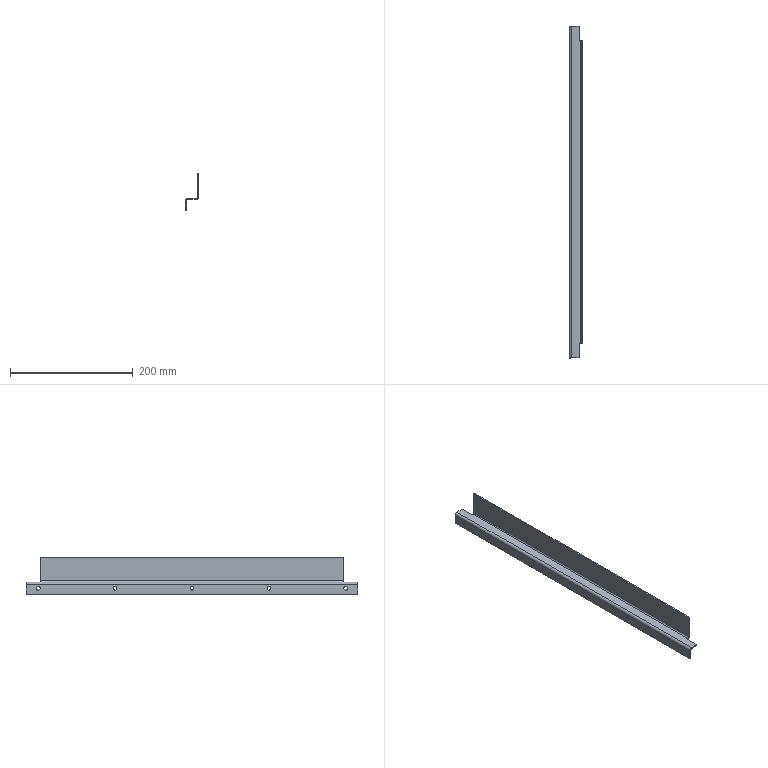Part | NX | features solid 2 | 1 solid | 28 faces | box 22 x 540 x 60 mm | volume 79205 mm3 | plane 14 | cylinder 14 | commonest cylinder face diameters 6 x10 4 x2 8 x2
STEP:
#1=CARTESIAN_POINT('',(-1090.,-1270.9,118.));
#2=VERTEX_POINT('',#1);
#3=CARTESIAN_POINT('',(-1092.,-1270.9,118.));
#4=VERTEX_POINT('',#3);
#5=CARTESIAN_POINT('',(-1108.,-1270.9,118.));
#6=DIRECTION('',(-1.,0.,0.));
#7=VECTOR('',#6,1000.);
#8=LINE('',#5,#7);
#9=EDGE_CURVE('',#2,#4,#8,.T.);
#10=ORIENTED_EDGE('',*,*,#9,.F.);
#11=CARTESIAN_POINT('',(-1086.,-1270.9,122.));
#12=VERTEX_POINT('',#11);
#13=CARTESIAN_POINT('',(-1090.,-1270.9,122.));
#14=DIRECTION('',(0.,1.,0.));
#15=DIRECTION('',(0.,0.,-1.));
#16=AXIS2_PLACEMENT_3D('',#13,#14,#15);
#17=CIRCLE('',#16,4.);
#18=EDGE_CURVE('',#12,#2,#17,.T.);
#19=ORIENTED_EDGE('',*,*,#18,.F.);
#20=CARTESIAN_POINT('',(-1086.,-1270.9,160.));
#21=VERTEX_POINT('',#20);
#22=CARTESIAN_POINT('',(-1086.,-1270.9,120.));
#23=DIRECTION('',(0.,0.,-1.));
#24=VECTOR('',#23,1000.);
#25=LINE('',#22,#24);
#26=EDGE_CURVE('',#21,#12,#25,.T.);
#27=ORIENTED_EDGE('',*,*,#26,.F.);
#28=CARTESIAN_POINT('',(-1088.,-1270.9,160.));
#29=VERTEX_POINT('',#28);
#30=CARTESIAN_POINT('',(-1088.,-1270.9,160.));
#31=DIRECTION('',(-1.,0.,0.));
#32=VECTOR('',#31,1000.);
#33=LINE('',#30,#32);
#34=EDGE_CURVE('',#21,#29,#33,.T.);
#35=ORIENTED_EDGE('',*,*,#34,.T.);
#36=CARTESIAN_POINT('',(-1088.,-1270.9,122.));
#37=VERTEX_POINT('',#36);
#38=CARTESIAN_POINT('',(-1088.,-1270.9,120.));
#39=DIRECTION('',(0.,0.,-1.));
#40=VECTOR('',#39,1000.);
#41=LINE('',#38,#40);
#42=EDGE_CURVE('',#29,#37,#41,.T.);
#43=ORIENTED_EDGE('',*,*,#42,.T.);
#44=CARTESIAN_POINT('',(-1090.,-1270.9,120.));
#45=VERTEX_POINT('',#44);
#46=CARTESIAN_POINT('',(-1090.,-1270.9,122.));
#47=DIRECTION('',(0.,1.,0.));
#48=DIRECTION('',(0.,0.,-1.));
#49=AXIS2_PLACEMENT_3D('',#46,#47,#48);
#50=CIRCLE('',#49,2.);
#51=EDGE_CURVE('',#37,#45,#50,.T.);
#52=ORIENTED_EDGE('',*,*,#51,.T.);
#53=CARTESIAN_POINT('',(-1092.,-1270.9,120.));
#54=VERTEX_POINT('',#53);
#55=CARTESIAN_POINT('',(-1108.,-1270.9,120.));
#56=DIRECTION('',(-1.,0.,0.));
#57=VECTOR('',#56,1000.);
#58=LINE('',#55,#57);
#59=EDGE_CURVE('',#45,#54,#58,.T.);
#60=ORIENTED_EDGE('',*,*,#59,.T.);
#61=CARTESIAN_POINT('',(-1092.,-1270.9,120.));
#62=DIRECTION('',(0.,0.,1.));
#63=VECTOR('',#62,1000.);
#64=LINE('',#61,#63);
#65=EDGE_CURVE('',#4,#54,#64,.T.);
#66=ORIENTED_EDGE('',*,*,#65,.F.);
#67=EDGE_LOOP('',(#10,#19,#27,#35,#43,#52,#60,#66));
#68=FACE_BOUND('',#67,.T.);
#69=CARTESIAN_POINT('',(-1108.,-1270.9,120.));
#70=DIRECTION('',(0.,1.,0.));
#71=DIRECTION('',(0.,0.,-1.));
#72=AXIS2_PLACEMENT_3D('',#69,#70,#71);
#73=PLANE('',#72);
#74=ADVANCED_FACE('',(#68),#73,.F.);
#75=ORIENTED_EDGE('',*,*,#65,.T.);
#76=CARTESIAN_POINT('',(-1092.,-1294.,120.));
#77=VERTEX_POINT('',#76);
#78=CARTESIAN_POINT('',(-1092.,-1294.,120.));
#79=DIRECTION('',(0.,1.,0.));
#80=VECTOR('',#79,1000.);
#81=LINE('',#78,#80);
#82=EDGE_CURVE('',#77,#54,#81,.T.);
#83=ORIENTED_EDGE('',*,*,#82,.F.);
#84=CARTESIAN_POINT('',(-1092.,-1294.,118.));
#85=VERTEX_POINT('',#84);
#86=CARTESIAN_POINT('',(-1092.,-1294.,120.));
#87=DIRECTION('',(0.,0.,1.));
#88=VECTOR('',#87,1000.);
#89=LINE('',#86,#88);
#90=EDGE_CURVE('',#85,#77,#89,.T.);
#91=ORIENTED_EDGE('',*,*,#90,.F.);
#92=CARTESIAN_POINT('',(-1092.,-1294.,118.));
#93=DIRECTION('',(0.,1.,0.));
#94=VECTOR('',#93,1000.);
#95=LINE('',#92,#94);
#96=EDGE_CURVE('',#85,#4,#95,.T.);
#97=ORIENTED_EDGE('',*,*,#96,.T.);
#98=EDGE_LOOP('',(#75,#83,#91,#97));
#99=FACE_BOUND('',#98,.T.);
#100=CARTESIAN_POINT('',(-1092.,-1294.,120.));
#101=DIRECTION('',(1.,0.,0.));
#102=DIRECTION('',(0.,0.,-1.));
#103=AXIS2_PLACEMENT_3D('',#100,#101,#102);
#104=PLANE('',#103);
#105=ADVANCED_FACE('',(#99),#104,.T.);
#106=CARTESIAN_POINT('',(-1086.,-777.1,122.));
#107=VERTEX_POINT('',#106);
#108=CARTESIAN_POINT('',(-1086.,-777.1,160.));
#109=VERTEX_POINT('',#108);
#110=CARTESIAN_POINT('',(-1086.,-777.1,120.));
#111=DIRECTION('',(0.,0.,1.));
#112=VECTOR('',#111,1000.);
#113=LINE('',#110,#112);
#114=EDGE_CURVE('',#107,#109,#113,.T.);
#115=ORIENTED_EDGE('',*,*,#114,.F.);
#116=CARTESIAN_POINT('',(-1090.,-777.1,118.));
#117=VERTEX_POINT('',#116);
#118=CARTESIAN_POINT('',(-1090.,-777.1,122.));
#119=DIRECTION('',(0.,-1.,0.));
#120=DIRECTION('',(0.,0.,-1.));
#121=AXIS2_PLACEMENT_3D('',#118,#119,#120);
#122=CIRCLE('',#121,4.);
#123=EDGE_CURVE('',#117,#107,#122,.T.);
#124=ORIENTED_EDGE('',*,*,#123,.F.);
#125=CARTESIAN_POINT('',(-1092.,-777.1,118.));
#126=VERTEX_POINT('',#125);
#127=CARTESIAN_POINT('',(-1108.,-777.1,118.));
#128=DIRECTION('',(1.,0.,0.));
#129=VECTOR('',#128,1000.);
#130=LINE('',#127,#129);
#131=EDGE_CURVE('',#126,#117,#130,.T.);
#132=ORIENTED_EDGE('',*,*,#131,.F.);
#133=CARTESIAN_POINT('',(-1092.,-777.1,120.));
#134=VERTEX_POINT('',#133);
#135=CARTESIAN_POINT('',(-1092.,-777.1,120.));
#136=DIRECTION('',(0.,0.,1.));
#137=VECTOR('',#136,1000.);
#138=LINE('',#135,#137);
#139=EDGE_CURVE('',#126,#134,#138,.T.);
#140=ORIENTED_EDGE('',*,*,#139,.T.);
#141=CARTESIAN_POINT('',(-1090.,-777.1,120.));
#142=VERTEX_POINT('',#141);
#143=CARTESIAN_POINT('',(-1108.,-777.1,120.));
#144=DIRECTION('',(1.,0.,0.));
#145=VECTOR('',#144,1000.);
#146=LINE('',#143,#145);
#147=EDGE_CURVE('',#134,#142,#146,.T.);
#148=ORIENTED_EDGE('',*,*,#147,.T.);
#149=CARTESIAN_POINT('',(-1088.,-777.1,122.));
#150=VERTEX_POINT('',#149);
#151=CARTESIAN_POINT('',(-1090.,-777.1,122.));
#152=DIRECTION('',(0.,-1.,0.));
#153=DIRECTION('',(0.,0.,1.));
#154=AXIS2_PLACEMENT_3D('',#151,#152,#153);
#155=CIRCLE('',#154,2.);
#156=EDGE_CURVE('',#142,#150,#155,.T.);
#157=ORIENTED_EDGE('',*,*,#156,.T.);
#158=CARTESIAN_POINT('',(-1088.,-777.1,160.));
#159=VERTEX_POINT('',#158);
#160=CARTESIAN_POINT('',(-1088.,-777.1,120.));
#161=DIRECTION('',(0.,0.,1.));
#162=VECTOR('',#161,1000.);
#163=LINE('',#160,#162);
#164=EDGE_CURVE('',#150,#159,#163,.T.);
#165=ORIENTED_EDGE('',*,*,#164,.T.);
#166=CARTESIAN_POINT('',(-1088.,-777.1,160.));
#167=DIRECTION('',(-1.,0.,0.));
#168=VECTOR('',#167,1000.);
#169=LINE('',#166,#168);
#170=EDGE_CURVE('',#109,#159,#169,.T.);
#171=ORIENTED_EDGE('',*,*,#170,.F.);
#172=EDGE_LOOP('',(#115,#124,#132,#140,#148,#157,#165,#171));
#173=FACE_BOUND('',#172,.T.);
#174=CARTESIAN_POINT('',(-1088.,-777.1,120.));
#175=DIRECTION('',(0.,-1.,0.));
#176=DIRECTION('',(-1.,0.,0.));
#177=AXIS2_PLACEMENT_3D('',#174,#175,#176);
#178=PLANE('',#177);
#179=ADVANCED_FACE('',(#173),#178,.F.);
#180=CARTESIAN_POINT('',(-1092.,-754.,118.));
#181=VERTEX_POINT('',#180);
#182=CARTESIAN_POINT('',(-1092.,-754.,120.));
#183=VERTEX_POINT('',#182);
#184=CARTESIAN_POINT('',(-1092.,-754.,120.));
#185=DIRECTION('',(0.,0.,1.));
#186=VECTOR('',#185,1000.);
#187=LINE('',#184,#186);
#188=EDGE_CURVE('',#181,#183,#187,.T.);
#189=ORIENTED_EDGE('',*,*,#188,.T.);
#190=CARTESIAN_POINT('',(-1092.,-1294.,120.));
#191=DIRECTION('',(0.,1.,0.));
#192=VECTOR('',#191,1000.);
#193=LINE('',#190,#192);
#194=EDGE_CURVE('',#134,#183,#193,.T.);
#195=ORIENTED_EDGE('',*,*,#194,.F.);
#196=ORIENTED_EDGE('',*,*,#139,.F.);
#197=CARTESIAN_POINT('',(-1092.,-1294.,118.));
#198=DIRECTION('',(0.,1.,0.));
#199=VECTOR('',#198,1000.);
#200=LINE('',#197,#199);
#201=EDGE_CURVE('',#126,#181,#200,.T.);
#202=ORIENTED_EDGE('',*,*,#201,.T.);
#203=EDGE_LOOP('',(#189,#195,#196,#202));
#204=FACE_BOUND('',#203,.T.);
#205=CARTESIAN_POINT('',(-1092.,-1294.,120.));
#206=DIRECTION('',(1.,0.,0.));
#207=DIRECTION('',(0.,0.,-1.));
#208=AXIS2_PLACEMENT_3D('',#205,#206,#207);
#209=PLANE('',#208);
#210=ADVANCED_FACE('',(#204),#209,.T.);
#211=CARTESIAN_POINT('',(-1108.,-1024.,107.));
#212=VERTEX_POINT('',#211);
#213=CARTESIAN_POINT('',(-1106.,-1024.,107.));
#214=VERTEX_POINT('',#213);
#215=CARTESIAN_POINT('',(-1649.768,-1024.,107.));
#216=DIRECTION('',(1.,0.,0.));
#217=VECTOR('',#216,1000.);
#218=LINE('',#215,#217);
#219=EDGE_CURVE('',#212,#214,#218,.T.);
#220=ORIENTED_EDGE('',*,*,#219,.F.);
#221=CARTESIAN_POINT('',(-1108.,-1024.,113.));
#222=VERTEX_POINT('',#221);
#223=CARTESIAN_POINT('',(-1108.,-1024.,110.));
#224=DIRECTION('',(-1.,0.,0.));
#225=DIRECTION('',(0.,0.,-1.));
#226=AXIS2_PLACEMENT_3D('',#223,#224,#225);
#227=CIRCLE('',#226,3.);
#228=EDGE_CURVE('',#212,#222,#227,.T.);
#229=ORIENTED_EDGE('',*,*,#228,.T.);
#230=CARTESIAN_POINT('',(-1106.,-1024.,113.));
#231=VERTEX_POINT('',#230);
#232=CARTESIAN_POINT('',(-1649.768,-1024.,113.));
#233=DIRECTION('',(1.,0.,0.));
#234=VECTOR('',#233,1000.);
#235=LINE('',#232,#234);
#236=EDGE_CURVE('',#231,#222,#235,.F.);
#237=ORIENTED_EDGE('',*,*,#236,.F.);
#238=CARTESIAN_POINT('',(-1106.,-1024.,110.));
#239=DIRECTION('',(1.,0.,0.));
#240=DIRECTION('',(0.,1.,0.));
#241=AXIS2_PLACEMENT_3D('',#238,#239,#240);
#242=CIRCLE('',#241,3.);
#243=EDGE_CURVE('',#231,#214,#242,.T.);
#244=ORIENTED_EDGE('',*,*,#243,.T.);
#245=EDGE_LOOP('',(#220,#229,#237,#244));
#246=FACE_BOUND('',#245,.T.);
#247=CARTESIAN_POINT('',(-1649.768,-1024.,110.));
#248=DIRECTION('',(1.,0.,0.));
#249=DIRECTION('',(0.,0.,1.));
#250=AXIS2_PLACEMENT_3D('',#247,#248,#249);
#251=CYLINDRICAL_SURFACE('',#250,3.);
#252=ADVANCED_FACE('',(#246),#251,.F.);
#253=CARTESIAN_POINT('',(-1108.,-1274.,107.));
#254=VERTEX_POINT('',#253);
#255=CARTESIAN_POINT('',(-1106.,-1274.,107.));
#256=VERTEX_POINT('',#255);
#257=CARTESIAN_POINT('',(-1649.768,-1274.,107.));
#258=DIRECTION('',(1.,0.,0.));
#259=VECTOR('',#258,1000.);
#260=LINE('',#257,#259);
#261=EDGE_CURVE('',#254,#256,#260,.T.);
#262=ORIENTED_EDGE('',*,*,#261,.F.);
#263=CARTESIAN_POINT('',(-1108.,-1274.,113.));
#264=VERTEX_POINT('',#263);
#265=CARTESIAN_POINT('',(-1108.,-1274.,110.));
#266=DIRECTION('',(-1.,0.,0.));
#267=DIRECTION('',(0.,0.,-1.));
#268=AXIS2_PLACEMENT_3D('',#265,#266,#267);
#269=CIRCLE('',#268,3.);
#270=EDGE_CURVE('',#254,#264,#269,.T.);
#271=ORIENTED_EDGE('',*,*,#270,.T.);
#272=CARTESIAN_POINT('',(-1106.,-1274.,113.));
#273=VERTEX_POINT('',#272);
#274=CARTESIAN_POINT('',(-1649.768,-1274.,113.));
#275=DIRECTION('',(1.,0.,0.));
#276=VECTOR('',#275,1000.);
#277=LINE('',#274,#276);
#278=EDGE_CURVE('',#273,#264,#277,.F.);
#279=ORIENTED_EDGE('',*,*,#278,.F.);
#280=CARTESIAN_POINT('',(-1106.,-1274.,110.));
#281=DIRECTION('',(1.,0.,0.));
#282=DIRECTION('',(0.,1.,0.));
#283=AXIS2_PLACEMENT_3D('',#280,#281,#282);
#284=CIRCLE('',#283,3.);
#285=EDGE_CURVE('',#273,#256,#284,.T.);
#286=ORIENTED_EDGE('',*,*,#285,.T.);
#287=EDGE_LOOP('',(#262,#271,#279,#286));
#288=FACE_BOUND('',#287,.T.);
#289=CARTESIAN_POINT('',(-1649.768,-1274.,110.));
#290=DIRECTION('',(1.,0.,0.));
#291=DIRECTION('',(0.,0.,1.));
#292=AXIS2_PLACEMENT_3D('',#289,#290,#291);
#293=CYLINDRICAL_SURFACE('',#292,3.);
#294=ADVANCED_FACE('',(#288),#293,.F.);
#295=CARTESIAN_POINT('',(-1106.,-1149.,107.));
#296=VERTEX_POINT('',#295);
#297=CARTESIAN_POINT('',(-1108.,-1149.,107.));
#298=VERTEX_POINT('',#297);
#299=CARTESIAN_POINT('',(-1649.768,-1149.,107.));
#300=DIRECTION('',(1.,0.,0.));
#301=VECTOR('',#300,1000.);
#302=LINE('',#299,#301);
#303=EDGE_CURVE('',#296,#298,#302,.F.);
#304=ORIENTED_EDGE('',*,*,#303,.T.);
#305=CARTESIAN_POINT('',(-1108.,-1149.,113.));
#306=VERTEX_POINT('',#305);
#307=CARTESIAN_POINT('',(-1108.,-1149.,110.));
#308=DIRECTION('',(-1.,0.,0.));
#309=DIRECTION('',(0.,0.,-1.));
#310=AXIS2_PLACEMENT_3D('',#307,#308,#309);
#311=CIRCLE('',#310,3.);
#312=EDGE_CURVE('',#298,#306,#311,.T.);
#313=ORIENTED_EDGE('',*,*,#312,.T.);
#314=CARTESIAN_POINT('',(-1106.,-1149.,113.));
#315=VERTEX_POINT('',#314);
#316=CARTESIAN_POINT('',(-1649.768,-1149.,113.));
#317=DIRECTION('',(1.,0.,0.));
#318=VECTOR('',#317,1000.);
#319=LINE('',#316,#318);
#320=EDGE_CURVE('',#306,#315,#319,.T.);
#321=ORIENTED_EDGE('',*,*,#320,.T.);
#322=CARTESIAN_POINT('',(-1106.,-1149.,110.));
#323=DIRECTION('',(1.,0.,0.));
#324=DIRECTION('',(0.,1.,0.));
#325=AXIS2_PLACEMENT_3D('',#322,#323,#324);
#326=CIRCLE('',#325,3.);
#327=EDGE_CURVE('',#315,#296,#326,.T.);
#328=ORIENTED_EDGE('',*,*,#327,.T.);
#329=EDGE_LOOP('',(#304,#313,#321,#328));
#330=FACE_BOUND('',#329,.T.);
#331=CARTESIAN_POINT('',(-1649.768,-1149.,110.));
#332=DIRECTION('',(1.,0.,0.));
#333=DIRECTION('',(0.,0.,1.));
#334=AXIS2_PLACEMENT_3D('',#331,#332,#333);
#335=CYLINDRICAL_SURFACE('',#334,3.);
#336=ADVANCED_FACE('',(#330),#335,.F.);
#337=CARTESIAN_POINT('',(-1108.,-774.,107.));
#338=VERTEX_POINT('',#337);
#339=CARTESIAN_POINT('',(-1106.,-774.,107.));
#340=VERTEX_POINT('',#339);
#341=CARTESIAN_POINT('',(-1649.768,-774.,107.));
#342=DIRECTION('',(1.,0.,0.));
#343=VECTOR('',#342,1000.);
#344=LINE('',#341,#343);
#345=EDGE_CURVE('',#338,#340,#344,.T.);
#346=ORIENTED_EDGE('',*,*,#345,.F.);
#347=CARTESIAN_POINT('',(-1108.,-774.,113.));
#348=VERTEX_POINT('',#347);
#349=CARTESIAN_POINT('',(-1108.,-774.,110.));
#350=DIRECTION('',(-1.,0.,0.));
#351=DIRECTION('',(0.,0.,-1.));
#352=AXIS2_PLACEMENT_3D('',#349,#350,#351);
#353=CIRCLE('',#352,3.);
#354=EDGE_CURVE('',#338,#348,#353,.T.);
#355=ORIENTED_EDGE('',*,*,#354,.T.);
#356=CARTESIAN_POINT('',(-1106.,-774.,113.));
#357=VERTEX_POINT('',#356);
#358=CARTESIAN_POINT('',(-1649.768,-774.,113.));
#359=DIRECTION('',(1.,0.,0.));
#360=VECTOR('',#359,1000.);
#361=LINE('',#358,#360);
#362=EDGE_CURVE('',#357,#348,#361,.F.);
#363=ORIENTED_EDGE('',*,*,#362,.F.);
#364=CARTESIAN_POINT('',(-1106.,-774.,110.));
#365=DIRECTION('',(1.,0.,0.));
#366=DIRECTION('',(0.,1.,0.));
#367=AXIS2_PLACEMENT_3D('',#364,#365,#366);
#368=CIRCLE('',#367,3.);
#369=EDGE_CURVE('',#357,#340,#368,.T.);
#370=ORIENTED_EDGE('',*,*,#369,.T.);
#371=EDGE_LOOP('',(#346,#355,#363,#370));
#372=FACE_BOUND('',#371,.T.);
#373=CARTESIAN_POINT('',(-1649.768,-774.,110.));
#374=DIRECTION('',(1.,0.,0.));
#375=DIRECTION('',(0.,0.,1.));
#376=AXIS2_PLACEMENT_3D('',#373,#374,#375);
#377=CYLINDRICAL_SURFACE('',#376,3.);
#378=ADVANCED_FACE('',(#372),#377,.F.);
#379=CARTESIAN_POINT('',(-1108.,-899.,107.));
#380=VERTEX_POINT('',#379);
#381=CARTESIAN_POINT('',(-1106.,-899.,107.));
#382=VERTEX_POINT('',#381);
#383=CARTESIAN_POINT('',(-1649.768,-899.,107.));
#384=DIRECTION('',(1.,0.,0.));
#385=VECTOR('',#384,1000.);
#386=LINE('',#383,#385);
#387=EDGE_CURVE('',#380,#382,#386,.T.);
#388=ORIENTED_EDGE('',*,*,#387,.F.);
#389=CARTESIAN_POINT('',(-1108.,-899.,113.));
#390=VERTEX_POINT('',#389);
#391=CARTESIAN_POINT('',(-1108.,-899.,110.));
#392=DIRECTION('',(-1.,0.,0.));
#393=DIRECTION('',(0.,0.,-1.));
#394=AXIS2_PLACEMENT_3D('',#391,#392,#393);
#395=CIRCLE('',#394,3.);
#396=EDGE_CURVE('',#380,#390,#395,.T.);
#397=ORIENTED_EDGE('',*,*,#396,.T.);
#398=CARTESIAN_POINT('',(-1106.,-899.,113.));
#399=VERTEX_POINT('',#398);
#400=CARTESIAN_POINT('',(-1649.768,-899.,113.));
#401=DIRECTION('',(1.,0.,0.));
#402=VECTOR('',#401,1000.);
#403=LINE('',#400,#402);
#404=EDGE_CURVE('',#399,#390,#403,.F.);
#405=ORIENTED_EDGE('',*,*,#404,.F.);
#406=CARTESIAN_POINT('',(-1106.,-899.,110.));
#407=DIRECTION('',(1.,0.,0.));
#408=DIRECTION('',(0.,1.,0.));
#409=AXIS2_PLACEMENT_3D('',#406,#407,#408);
#410=CIRCLE('',#409,3.);
#411=EDGE_CURVE('',#399,#382,#410,.T.);
#412=ORIENTED_EDGE('',*,*,#411,.T.);
#413=EDGE_LOOP('',(#388,#397,#405,#412));
#414=FACE_BOUND('',#413,.T.);
#415=CARTESIAN_POINT('',(-1649.768,-899.,110.));
#416=DIRECTION('',(1.,0.,0.));
#417=DIRECTION('',(0.,0.,1.));
#418=AXIS2_PLACEMENT_3D('',#415,#416,#417);
#419=CYLINDRICAL_SURFACE('',#418,3.);
#420=ADVANCED_FACE('',(#414),#419,.F.);
#421=CARTESIAN_POINT('',(-1086.,-1294.,160.));
#422=DIRECTION('',(0.,1.,0.));
#423=VECTOR('',#422,1000.);
#424=LINE('',#421,#423);
#425=EDGE_CURVE('',#21,#109,#424,.T.);
#426=ORIENTED_EDGE('',*,*,#425,.F.);
#427=ORIENTED_EDGE('',*,*,#26,.T.);
#428=CARTESIAN_POINT('',(-1086.,-1294.,122.));
#429=DIRECTION('',(0.,1.,0.));
#430=VECTOR('',#429,1000.);
#431=LINE('',#428,#430);
#432=EDGE_CURVE('',#12,#107,#431,.T.);
#433=ORIENTED_EDGE('',*,*,#432,.T.);
#434=ORIENTED_EDGE('',*,*,#114,.T.);
#435=EDGE_LOOP('',(#426,#427,#433,#434));
#436=FACE_BOUND('',#435,.T.);
#437=CARTESIAN_POINT('',(-1086.,-1294.,120.));
#438=DIRECTION('',(-1.,0.,0.));
#439=DIRECTION('',(0.,1.,0.));
#440=AXIS2_PLACEMENT_3D('',#437,#438,#439);
#441=PLANE('',#440);
#442=ADVANCED_FACE('',(#436),#441,.F.);
#443=ORIENTED_EDGE('',*,*,#432,.F.);
#444=ORIENTED_EDGE('',*,*,#18,.T.);
#445=CARTESIAN_POINT('',(-1090.,-1294.,118.));
#446=DIRECTION('',(0.,1.,0.));
#447=VECTOR('',#446,1000.);
#448=LINE('',#445,#447);
#449=EDGE_CURVE('',#2,#117,#448,.T.);
#450=ORIENTED_EDGE('',*,*,#449,.T.);
#451=ORIENTED_EDGE('',*,*,#123,.T.);
#452=EDGE_LOOP('',(#443,#444,#450,#451));
#453=FACE_BOUND('',#452,.T.);
#454=CARTESIAN_POINT('',(-1090.,-1294.,122.));
#455=DIRECTION('',(0.,1.,0.));
#456=DIRECTION('',(0.,0.,-1.));
#457=AXIS2_PLACEMENT_3D('',#454,#455,#456);
#458=CYLINDRICAL_SURFACE('',#457,4.);
#459=ADVANCED_FACE('',(#453),#458,.T.);
#460=ORIENTED_EDGE('',*,*,#9,.T.);
#461=ORIENTED_EDGE('',*,*,#96,.F.);
#462=CARTESIAN_POINT('',(-1104.,-1294.,118.));
#463=VERTEX_POINT('',#462);
#464=CARTESIAN_POINT('',(-1108.,-1294.,118.));
#465=DIRECTION('',(1.,0.,0.));
#466=VECTOR('',#465,1000.);
#467=LINE('',#464,#466);
#468=EDGE_CURVE('',#463,#85,#467,.T.);
#469=ORIENTED_EDGE('',*,*,#468,.F.);
#470=CARTESIAN_POINT('',(-1104.,-754.,118.));
#471=VERTEX_POINT('',#470);
#472=CARTESIAN_POINT('',(-1104.,-1294.,118.));
#473=DIRECTION('',(0.,1.,0.));
#474=VECTOR('',#473,1000.);
#475=LINE('',#472,#474);
#476=EDGE_CURVE('',#463,#471,#475,.T.);
#477=ORIENTED_EDGE('',*,*,#476,.T.);
#478=CARTESIAN_POINT('',(-1108.,-754.,118.));
#479=DIRECTION('',(1.,0.,0.));
#480=VECTOR('',#479,1000.);
#481=LINE('',#478,#480);
#482=EDGE_CURVE('',#471,#181,#481,.T.);
#483=ORIENTED_EDGE('',*,*,#482,.T.);
#484=ORIENTED_EDGE('',*,*,#201,.F.);
#485=ORIENTED_EDGE('',*,*,#131,.T.);
#486=ORIENTED_EDGE('',*,*,#449,.F.);
#487=EDGE_LOOP('',(#460,#461,#469,#477,#483,#484,#485,#486));
#488=FACE_BOUND('',#487,.T.);
#489=CARTESIAN_POINT('',(-1108.,-1294.,118.));
#490=DIRECTION('',(0.,0.,1.));
#491=DIRECTION('',(0.,-1.,0.));
#492=AXIS2_PLACEMENT_3D('',#489,#490,#491);
#493=PLANE('',#492);
#494=ADVANCED_FACE('',(#488),#493,.F.);
#495=CARTESIAN_POINT('',(-1106.,-754.,116.));
#496=VERTEX_POINT('',#495);
#497=CARTESIAN_POINT('',(-1104.,-754.,116.));
#498=DIRECTION('',(0.,1.,0.));
#499=DIRECTION('',(0.,0.,-1.));
#500=AXIS2_PLACEMENT_3D('',#497,#498,#499);
#501=CIRCLE('',#500,2.);
#502=EDGE_CURVE('',#496,#471,#501,.T.);
#503=ORIENTED_EDGE('',*,*,#502,.T.);
#504=ORIENTED_EDGE('',*,*,#476,.F.);
#505=CARTESIAN_POINT('',(-1106.,-1294.,116.));
#506=VERTEX_POINT('',#505);
#507=CARTESIAN_POINT('',(-1104.,-1294.,116.));
#508=DIRECTION('',(0.,1.,0.));
#509=DIRECTION('',(0.,0.,-1.));
#510=AXIS2_PLACEMENT_3D('',#507,#508,#509);
#511=CIRCLE('',#510,2.);
#512=EDGE_CURVE('',#506,#463,#511,.T.);
#513=ORIENTED_EDGE('',*,*,#512,.F.);
#514=CARTESIAN_POINT('',(-1106.,-1294.,116.));
#515=DIRECTION('',(0.,1.,0.));
#516=VECTOR('',#515,1000.);
#517=LINE('',#514,#516);
#518=EDGE_CURVE('',#506,#496,#517,.T.);
#519=ORIENTED_EDGE('',*,*,#518,.T.);
#520=EDGE_LOOP('',(#503,#504,#513,#519));
#521=FACE_BOUND('',#520,.T.);
#522=CARTESIAN_POINT('',(-1104.,-1294.,116.));
#523=DIRECTION('',(0.,1.,0.));
#524=DIRECTION('',(0.,0.,-1.));
#525=AXIS2_PLACEMENT_3D('',#522,#523,#524);
#526=CYLINDRICAL_SURFACE('',#525,2.);
#527=ADVANCED_FACE('',(#521),#526,.F.);
#528=ORIENTED_EDGE('',*,*,#411,.F.);
#529=CARTESIAN_POINT('',(-1106.,-899.,110.));
#530=DIRECTION('',(1.,0.,0.));
#531=DIRECTION('',(0.,1.,0.));
#532=AXIS2_PLACEMENT_3D('',#529,#530,#531);
#533=CIRCLE('',#532,3.);
#534=EDGE_CURVE('',#382,#399,#533,.T.);
#535=ORIENTED_EDGE('',*,*,#534,.F.);
#536=EDGE_LOOP('',(#528,#535));
#537=FACE_BOUND('',#536,.T.);
#538=ORIENTED_EDGE('',*,*,#369,.F.);
#539=CARTESIAN_POINT('',(-1106.,-774.,110.));
#540=DIRECTION('',(1.,0.,0.));
#541=DIRECTION('',(0.,1.,0.));
#542=AXIS2_PLACEMENT_3D('',#539,#540,#541);
#543=CIRCLE('',#542,3.);
#544=EDGE_CURVE('',#340,#357,#543,.T.);
#545=ORIENTED_EDGE('',*,*,#544,.F.);
#546=EDGE_LOOP('',(#538,#545));
#547=FACE_BOUND('',#546,.T.);
#548=ORIENTED_EDGE('',*,*,#327,.F.);
#549=CARTESIAN_POINT('',(-1106.,-1149.,110.));
#550=DIRECTION('',(1.,0.,0.));
#551=DIRECTION('',(0.,1.,0.));
#552=AXIS2_PLACEMENT_3D('',#549,#550,#551);
#553=CIRCLE('',#552,3.);
#554=EDGE_CURVE('',#296,#315,#553,.T.);
#555=ORIENTED_EDGE('',*,*,#554,.F.);
#556=EDGE_LOOP('',(#548,#555));
#557=FACE_BOUND('',#556,.T.);
#558=ORIENTED_EDGE('',*,*,#285,.F.);
#559=CARTESIAN_POINT('',(-1106.,-1274.,110.));
#560=DIRECTION('',(1.,0.,0.));
#561=DIRECTION('',(0.,1.,0.));
#562=AXIS2_PLACEMENT_3D('',#559,#560,#561);
#563=CIRCLE('',#562,3.);
#564=EDGE_CURVE('',#256,#273,#563,.T.);
#565=ORIENTED_EDGE('',*,*,#564,.F.);
#566=EDGE_LOOP('',(#558,#565));
#567=FACE_BOUND('',#566,.T.);
#568=ORIENTED_EDGE('',*,*,#243,.F.);
#569=CARTESIAN_POINT('',(-1106.,-1024.,110.));
#570=DIRECTION('',(1.,0.,0.));
#571=DIRECTION('',(0.,1.,0.));
#572=AXIS2_PLACEMENT_3D('',#569,#570,#571);
#573=CIRCLE('',#572,3.);
#574=EDGE_CURVE('',#214,#231,#573,.T.);
#575=ORIENTED_EDGE('',*,*,#574,.F.);
#576=EDGE_LOOP('',(#568,#575));
#577=FACE_BOUND('',#576,.T.);
#578=CARTESIAN_POINT('',(-1106.,-754.,100.));
#579=VERTEX_POINT('',#578);
#580=CARTESIAN_POINT('',(-1106.,-754.,100.));
#581=DIRECTION('',(0.,0.,1.));
#582=VECTOR('',#581,1000.);
#583=LINE('',#580,#582);
#584=EDGE_CURVE('',#579,#496,#583,.T.);
#585=ORIENTED_EDGE('',*,*,#584,.T.);
#586=ORIENTED_EDGE('',*,*,#518,.F.);
#587=CARTESIAN_POINT('',(-1106.,-1294.,100.));
#588=VERTEX_POINT('',#587);
#589=CARTESIAN_POINT('',(-1106.,-1294.,100.));
#590=DIRECTION('',(0.,0.,1.));
#591=VECTOR('',#590,1000.);
#592=LINE('',#589,#591);
#593=EDGE_CURVE('',#588,#506,#592,.T.);
#594=ORIENTED_EDGE('',*,*,#593,.F.);
#595=CARTESIAN_POINT('',(-1106.,-1294.,100.));
#596=DIRECTION('',(0.,1.,0.));
#597=VECTOR('',#596,1000.);
#598=LINE('',#595,#597);
#599=EDGE_CURVE('',#588,#579,#598,.T.);
#600=ORIENTED_EDGE('',*,*,#599,.T.);
#601=EDGE_LOOP('',(#585,#586,#594,#600));
#602=FACE_BOUND('',#601,.T.);
#603=CARTESIAN_POINT('',(-1106.,-1294.,100.));
#604=DIRECTION('',(-1.,0.,0.));
#605=DIRECTION('',(0.,1.,0.));
#606=AXIS2_PLACEMENT_3D('',#603,#604,#605);
#607=PLANE('',#606);
#608=ADVANCED_FACE('',(#537,#547,#557,#567,#577,#602),#607,.F.);
#609=ORIENTED_EDGE('',*,*,#42,.F.);
#610=CARTESIAN_POINT('',(-1088.,-1294.,160.));
#611=DIRECTION('',(0.,1.,0.));
#612=VECTOR('',#611,1000.);
#613=LINE('',#610,#612);
#614=EDGE_CURVE('',#29,#159,#613,.T.);
#615=ORIENTED_EDGE('',*,*,#614,.T.);
#616=ORIENTED_EDGE('',*,*,#164,.F.);
#617=CARTESIAN_POINT('',(-1088.,-1294.,122.));
#618=DIRECTION('',(0.,1.,0.));
#619=VECTOR('',#618,1000.);
#620=LINE('',#617,#619);
#621=EDGE_CURVE('',#37,#150,#620,.T.);
#622=ORIENTED_EDGE('',*,*,#621,.F.);
#623=EDGE_LOOP('',(#609,#615,#616,#622));
#624=FACE_BOUND('',#623,.T.);
#625=CARTESIAN_POINT('',(-1088.,-1294.,120.));
#626=DIRECTION('',(-1.,0.,0.));
#627=DIRECTION('',(0.,1.,0.));
#628=AXIS2_PLACEMENT_3D('',#625,#626,#627);
#629=PLANE('',#628);
#630=ADVANCED_FACE('',(#624),#629,.T.);
#631=ORIENTED_EDGE('',*,*,#51,.F.);
#632=ORIENTED_EDGE('',*,*,#621,.T.);
#633=ORIENTED_EDGE('',*,*,#156,.F.);
#634=CARTESIAN_POINT('',(-1090.,-1294.,120.));
#635=DIRECTION('',(0.,1.,0.));
#636=VECTOR('',#635,1000.);
#637=LINE('',#634,#636);
#638=EDGE_CURVE('',#45,#142,#637,.T.);
#639=ORIENTED_EDGE('',*,*,#638,.F.);
#640=EDGE_LOOP('',(#631,#632,#633,#639));
#641=FACE_BOUND('',#640,.T.);
#642=CARTESIAN_POINT('',(-1090.,-1294.,122.));
#643=DIRECTION('',(0.,1.,0.));
#644=DIRECTION('',(0.,0.,-1.));
#645=AXIS2_PLACEMENT_3D('',#642,#643,#644);
#646=CYLINDRICAL_SURFACE('',#645,2.);
#647=ADVANCED_FACE('',(#641),#646,.F.);
#648=ORIENTED_EDGE('',*,*,#82,.T.);
#649=ORIENTED_EDGE('',*,*,#59,.F.);
#650=ORIENTED_EDGE('',*,*,#638,.T.);
#651=ORIENTED_EDGE('',*,*,#147,.F.);
#652=ORIENTED_EDGE('',*,*,#194,.T.);
#653=CARTESIAN_POINT('',(-1104.,-754.,120.));
#654=VERTEX_POINT('',#653);
#655=CARTESIAN_POINT('',(-1108.,-754.,120.));
#656=DIRECTION('',(1.,0.,0.));
#657=VECTOR('',#656,1000.);
#658=LINE('',#655,#657);
#659=EDGE_CURVE('',#654,#183,#658,.T.);
#660=ORIENTED_EDGE('',*,*,#659,.F.);
#661=CARTESIAN_POINT('',(-1104.,-1294.,120.));
#662=VERTEX_POINT('',#661);
#663=CARTESIAN_POINT('',(-1104.,-1294.,120.));
#664=DIRECTION('',(0.,1.,0.));
#665=VECTOR('',#664,1000.);
#666=LINE('',#663,#665);
#667=EDGE_CURVE('',#662,#654,#666,.T.);
#668=ORIENTED_EDGE('',*,*,#667,.F.);
#669=CARTESIAN_POINT('',(-1108.,-1294.,120.));
#670=DIRECTION('',(1.,0.,0.));
#671=VECTOR('',#670,1000.);
#672=LINE('',#669,#671);
#673=EDGE_CURVE('',#662,#77,#672,.T.);
#674=ORIENTED_EDGE('',*,*,#673,.T.);
#675=EDGE_LOOP('',(#648,#649,#650,#651,#652,#660,#668,#674));
#676=FACE_BOUND('',#675,.T.);
#677=CARTESIAN_POINT('',(-1108.,-1294.,120.));
#678=DIRECTION('',(0.,0.,1.));
#679=DIRECTION('',(0.,-1.,0.));
#680=AXIS2_PLACEMENT_3D('',#677,#678,#679);
#681=PLANE('',#680);
#682=ADVANCED_FACE('',(#676),#681,.T.);
#683=CARTESIAN_POINT('',(-1108.,-754.,116.));
#684=VERTEX_POINT('',#683);
#685=CARTESIAN_POINT('',(-1104.,-754.,116.));
#686=DIRECTION('',(0.,1.,0.));
#687=DIRECTION('',(0.,0.,1.));
#688=AXIS2_PLACEMENT_3D('',#685,#686,#687);
#689=CIRCLE('',#688,4.);
#690=EDGE_CURVE('',#684,#654,#689,.T.);
#691=ORIENTED_EDGE('',*,*,#690,.F.);
#692=CARTESIAN_POINT('',(-1108.,-1294.,116.));
#693=VERTEX_POINT('',#692);
#694=CARTESIAN_POINT('',(-1108.,-1294.,116.));
#695=DIRECTION('',(0.,1.,0.));
#696=VECTOR('',#695,1000.);
#697=LINE('',#694,#696);
#698=EDGE_CURVE('',#693,#684,#697,.T.);
#699=ORIENTED_EDGE('',*,*,#698,.F.);
#700=CARTESIAN_POINT('',(-1104.,-1294.,116.));
#701=DIRECTION('',(0.,1.,0.));
#702=DIRECTION('',(0.,0.,1.));
#703=AXIS2_PLACEMENT_3D('',#700,#701,#702);
#704=CIRCLE('',#703,4.);
#705=EDGE_CURVE('',#693,#662,#704,.T.);
#706=ORIENTED_EDGE('',*,*,#705,.T.);
#707=ORIENTED_EDGE('',*,*,#667,.T.);
#708=EDGE_LOOP('',(#691,#699,#706,#707));
#709=FACE_BOUND('',#708,.T.);
#710=CARTESIAN_POINT('',(-1104.,-1294.,116.));
#711=DIRECTION('',(0.,1.,0.));
#712=DIRECTION('',(0.,0.,-1.));
#713=AXIS2_PLACEMENT_3D('',#710,#711,#712);
#714=CYLINDRICAL_SURFACE('',#713,4.);
#715=ADVANCED_FACE('',(#709),#714,.T.);
#716=CARTESIAN_POINT('',(-1108.,-899.,110.));
#717=DIRECTION('',(-1.,0.,0.));
#718=DIRECTION('',(0.,0.,-1.));
#719=AXIS2_PLACEMENT_3D('',#716,#717,#718);
#720=CIRCLE('',#719,3.);
#721=EDGE_CURVE('',#390,#380,#720,.T.);
#722=ORIENTED_EDGE('',*,*,#721,.F.);
#723=ORIENTED_EDGE('',*,*,#396,.F.);
#724=EDGE_LOOP('',(#722,#723));
#725=FACE_BOUND('',#724,.T.);
#726=CARTESIAN_POINT('',(-1108.,-774.,110.));
#727=DIRECTION('',(-1.,0.,0.));
#728=DIRECTION('',(0.,0.,-1.));
#729=AXIS2_PLACEMENT_3D('',#726,#727,#728);
#730=CIRCLE('',#729,3.);
#731=EDGE_CURVE('',#348,#338,#730,.T.);
#732=ORIENTED_EDGE('',*,*,#731,.F.);
#733=ORIENTED_EDGE('',*,*,#354,.F.);
#734=EDGE_LOOP('',(#732,#733));
#735=FACE_BOUND('',#734,.T.);
#736=CARTESIAN_POINT('',(-1108.,-1149.,110.));
#737=DIRECTION('',(-1.,0.,0.));
#738=DIRECTION('',(0.,0.,-1.));
#739=AXIS2_PLACEMENT_3D('',#736,#737,#738);
#740=CIRCLE('',#739,3.);
#741=EDGE_CURVE('',#306,#298,#740,.T.);
#742=ORIENTED_EDGE('',*,*,#741,.F.);
#743=ORIENTED_EDGE('',*,*,#312,.F.);
#744=EDGE_LOOP('',(#742,#743));
#745=FACE_BOUND('',#744,.T.);
#746=CARTESIAN_POINT('',(-1108.,-1274.,110.));
#747=DIRECTION('',(-1.,0.,0.));
#748=DIRECTION('',(0.,0.,-1.));
#749=AXIS2_PLACEMENT_3D('',#746,#747,#748);
#750=CIRCLE('',#749,3.);
#751=EDGE_CURVE('',#264,#254,#750,.T.);
#752=ORIENTED_EDGE('',*,*,#751,.F.);
#753=ORIENTED_EDGE('',*,*,#270,.F.);
#754=EDGE_LOOP('',(#752,#753));
#755=FACE_BOUND('',#754,.T.);
#756=CARTESIAN_POINT('',(-1108.,-1024.,110.));
#757=DIRECTION('',(-1.,0.,0.));
#758=DIRECTION('',(0.,0.,-1.));
#759=AXIS2_PLACEMENT_3D('',#756,#757,#758);
#760=CIRCLE('',#759,3.);
#761=EDGE_CURVE('',#222,#212,#760,.T.);
#762=ORIENTED_EDGE('',*,*,#761,.F.);
#763=ORIENTED_EDGE('',*,*,#228,.F.);
#764=EDGE_LOOP('',(#762,#763));
#765=FACE_BOUND('',#764,.T.);
#766=CARTESIAN_POINT('',(-1108.,-754.,100.));
#767=VERTEX_POINT('',#766);
#768=CARTESIAN_POINT('',(-1108.,-754.,100.));
#769=DIRECTION('',(0.,0.,1.));
#770=VECTOR('',#769,1000.);
#771=LINE('',#768,#770);
#772=EDGE_CURVE('',#767,#684,#771,.T.);
#773=ORIENTED_EDGE('',*,*,#772,.F.);
#774=CARTESIAN_POINT('',(-1108.,-1294.,100.));
#775=VERTEX_POINT('',#774);
#776=CARTESIAN_POINT('',(-1108.,-1294.,100.));
#777=DIRECTION('',(0.,1.,0.));
#778=VECTOR('',#777,1000.);
#779=LINE('',#776,#778);
#780=EDGE_CURVE('',#775,#767,#779,.T.);
#781=ORIENTED_EDGE('',*,*,#780,.F.);
#782=CARTESIAN_POINT('',(-1108.,-1294.,100.));
#783=DIRECTION('',(0.,0.,1.));
#784=VECTOR('',#783,1000.);
#785=LINE('',#782,#784);
#786=EDGE_CURVE('',#775,#693,#785,.T.);
#787=ORIENTED_EDGE('',*,*,#786,.T.);
#788=ORIENTED_EDGE('',*,*,#698,.T.);
#789=EDGE_LOOP('',(#773,#781,#787,#788));
#790=FACE_BOUND('',#789,.T.);
#791=CARTESIAN_POINT('',(-1108.,-1294.,100.));
#792=DIRECTION('',(-1.,0.,0.));
#793=DIRECTION('',(0.,1.,0.));
#794=AXIS2_PLACEMENT_3D('',#791,#792,#793);
#795=PLANE('',#794);
#796=ADVANCED_FACE('',(#725,#735,#745,#755,#765,#790),#795,.T.);
#797=ORIENTED_EDGE('',*,*,#599,.F.);
#798=CARTESIAN_POINT('',(-1108.,-1294.,100.));
#799=DIRECTION('',(-1.,0.,0.));
#800=VECTOR('',#799,1000.);
#801=LINE('',#798,#800);
#802=EDGE_CURVE('',#588,#775,#801,.T.);
#803=ORIENTED_EDGE('',*,*,#802,.T.);
#804=ORIENTED_EDGE('',*,*,#780,.T.);
#805=CARTESIAN_POINT('',(-1108.,-754.,100.));
#806=DIRECTION('',(-1.,0.,0.));
#807=VECTOR('',#806,1000.);
#808=LINE('',#805,#807);
#809=EDGE_CURVE('',#579,#767,#808,.T.);
#810=ORIENTED_EDGE('',*,*,#809,.F.);
#811=EDGE_LOOP('',(#797,#803,#804,#810));
#812=FACE_BOUND('',#811,.T.);
#813=CARTESIAN_POINT('',(-1108.,-1294.,100.));
#814=DIRECTION('',(0.,0.,1.));
#815=DIRECTION('',(0.,-1.,0.));
#816=AXIS2_PLACEMENT_3D('',#813,#814,#815);
#817=PLANE('',#816);
#818=ADVANCED_FACE('',(#812),#817,.F.);
#819=ORIENTED_EDGE('',*,*,#188,.F.);
#820=ORIENTED_EDGE('',*,*,#482,.F.);
#821=ORIENTED_EDGE('',*,*,#502,.F.);
#822=ORIENTED_EDGE('',*,*,#584,.F.);
#823=ORIENTED_EDGE('',*,*,#809,.T.);
#824=ORIENTED_EDGE('',*,*,#772,.T.);
#825=ORIENTED_EDGE('',*,*,#690,.T.);
#826=ORIENTED_EDGE('',*,*,#659,.T.);
#827=EDGE_LOOP('',(#819,#820,#821,#822,#823,#824,#825,#826));
#828=FACE_BOUND('',#827,.T.);
#829=CARTESIAN_POINT('',(-1108.,-754.,100.));
#830=DIRECTION('',(0.,-1.,0.));
#831=DIRECTION('',(-1.,0.,0.));
#832=AXIS2_PLACEMENT_3D('',#829,#830,#831);
#833=PLANE('',#832);
#834=ADVANCED_FACE('',(#828),#833,.F.);
#835=ORIENTED_EDGE('',*,*,#34,.F.);
#836=ORIENTED_EDGE('',*,*,#425,.T.);
#837=ORIENTED_EDGE('',*,*,#170,.T.);
#838=ORIENTED_EDGE('',*,*,#614,.F.);
#839=EDGE_LOOP('',(#835,#836,#837,#838));
#840=FACE_BOUND('',#839,.T.);
#841=CARTESIAN_POINT('',(-1088.,-1294.,160.));
#842=DIRECTION('',(0.,0.,1.));
#843=DIRECTION('',(0.,-1.,0.));
#844=AXIS2_PLACEMENT_3D('',#841,#842,#843);
#845=PLANE('',#844);
#846=ADVANCED_FACE('',(#840),#845,.T.);
#847=ORIENTED_EDGE('',*,*,#468,.T.);
#848=ORIENTED_EDGE('',*,*,#90,.T.);
#849=ORIENTED_EDGE('',*,*,#673,.F.);
#850=ORIENTED_EDGE('',*,*,#705,.F.);
#851=ORIENTED_EDGE('',*,*,#786,.F.);
#852=ORIENTED_EDGE('',*,*,#802,.F.);
#853=ORIENTED_EDGE('',*,*,#593,.T.);
#854=ORIENTED_EDGE('',*,*,#512,.T.);
#855=EDGE_LOOP('',(#847,#848,#849,#850,#851,#852,#853,#854));
#856=FACE_BOUND('',#855,.T.);
#857=CARTESIAN_POINT('',(-1088.,-1294.,120.));
#858=DIRECTION('',(0.,-1.,0.));
#859=DIRECTION('',(-1.,0.,0.));
#860=AXIS2_PLACEMENT_3D('',#857,#858,#859);
#861=PLANE('',#860);
#862=ADVANCED_FACE('',(#856),#861,.T.);
#863=ORIENTED_EDGE('',*,*,#721,.T.);
#864=ORIENTED_EDGE('',*,*,#387,.T.);
#865=ORIENTED_EDGE('',*,*,#534,.T.);
#866=ORIENTED_EDGE('',*,*,#404,.T.);
#867=EDGE_LOOP('',(#863,#864,#865,#866));
#868=FACE_BOUND('',#867,.T.);
#869=CARTESIAN_POINT('',(-1649.768,-899.,110.));
#870=DIRECTION('',(1.,0.,0.));
#871=DIRECTION('',(0.,0.,1.));
#872=AXIS2_PLACEMENT_3D('',#869,#870,#871);
#873=CYLINDRICAL_SURFACE('',#872,3.);
#874=ADVANCED_FACE('',(#868),#873,.F.);
#875=ORIENTED_EDGE('',*,*,#731,.T.);
#876=ORIENTED_EDGE('',*,*,#345,.T.);
#877=ORIENTED_EDGE('',*,*,#544,.T.);
#878=ORIENTED_EDGE('',*,*,#362,.T.);
#879=EDGE_LOOP('',(#875,#876,#877,#878));
#880=FACE_BOUND('',#879,.T.);
#881=CARTESIAN_POINT('',(-1649.768,-774.,110.));
#882=DIRECTION('',(1.,0.,0.));
#883=DIRECTION('',(0.,0.,1.));
#884=AXIS2_PLACEMENT_3D('',#881,#882,#883);
#885=CYLINDRICAL_SURFACE('',#884,3.);
#886=ADVANCED_FACE('',(#880),#885,.F.);
#887=ORIENTED_EDGE('',*,*,#741,.T.);
#888=ORIENTED_EDGE('',*,*,#303,.F.);
#889=ORIENTED_EDGE('',*,*,#554,.T.);
#890=ORIENTED_EDGE('',*,*,#320,.F.);
#891=EDGE_LOOP('',(#887,#888,#889,#890));
#892=FACE_BOUND('',#891,.T.);
#893=CARTESIAN_POINT('',(-1649.768,-1149.,110.));
#894=DIRECTION('',(1.,0.,0.));
#895=DIRECTION('',(0.,0.,1.));
#896=AXIS2_PLACEMENT_3D('',#893,#894,#895);
#897=CYLINDRICAL_SURFACE('',#896,3.);
#898=ADVANCED_FACE('',(#892),#897,.F.);
#899=ORIENTED_EDGE('',*,*,#751,.T.);
#900=ORIENTED_EDGE('',*,*,#261,.T.);
#901=ORIENTED_EDGE('',*,*,#564,.T.);
#902=ORIENTED_EDGE('',*,*,#278,.T.);
#903=EDGE_LOOP('',(#899,#900,#901,#902));
#904=FACE_BOUND('',#903,.T.);
#905=CARTESIAN_POINT('',(-1649.768,-1274.,110.));
#906=DIRECTION('',(1.,0.,0.));
#907=DIRECTION('',(0.,0.,1.));
#908=AXIS2_PLACEMENT_3D('',#905,#906,#907);
#909=CYLINDRICAL_SURFACE('',#908,3.);
#910=ADVANCED_FACE('',(#904),#909,.F.);
#911=ORIENTED_EDGE('',*,*,#761,.T.);
#912=ORIENTED_EDGE('',*,*,#219,.T.);
#913=ORIENTED_EDGE('',*,*,#574,.T.);
#914=ORIENTED_EDGE('',*,*,#236,.T.);
#915=EDGE_LOOP('',(#911,#912,#913,#914));
#916=FACE_BOUND('',#915,.T.);
#917=CARTESIAN_POINT('',(-1649.768,-1024.,110.));
#918=DIRECTION('',(1.,0.,0.));
#919=DIRECTION('',(0.,0.,1.));
#920=AXIS2_PLACEMENT_3D('',#917,#918,#919);
#921=CYLINDRICAL_SURFACE('',#920,3.);
#922=ADVANCED_FACE('',(#916),#921,.F.);
#923=CLOSED_SHELL('',(#74,#105,#179,#210,#252,#294,#336,#378,#420,#442,#459,#494,#527,#608,#630,#647,#682,#715,#796,#818,#834,#846,#862,#874,#886,#898,#910,#922));
#924=MANIFOLD_SOLID_BREP('',#923);
#925=(LENGTH_UNIT()NAMED_UNIT(*)SI_UNIT(.MILLI.,.METRE.));
#926=UNCERTAINTY_MEASURE_WITH_UNIT(LENGTH_MEASURE(0.00001),#925,'','');
#927=(NAMED_UNIT(*)PLANE_ANGLE_UNIT()SI_UNIT($,.RADIAN.));
#928=(NAMED_UNIT(*)SI_UNIT($,.STERADIAN.)SOLID_ANGLE_UNIT());
#929=(GEOMETRIC_REPRESENTATION_CONTEXT(3)GLOBAL_UNCERTAINTY_ASSIGNED_CONTEXT((#926))GLOBAL_UNIT_ASSIGNED_CONTEXT((#925,#927,#928))REPRESENTATION_CONTEXT('',''));
#930=ADVANCED_BREP_SHAPE_REPRESENTATION('',(#924),#929);